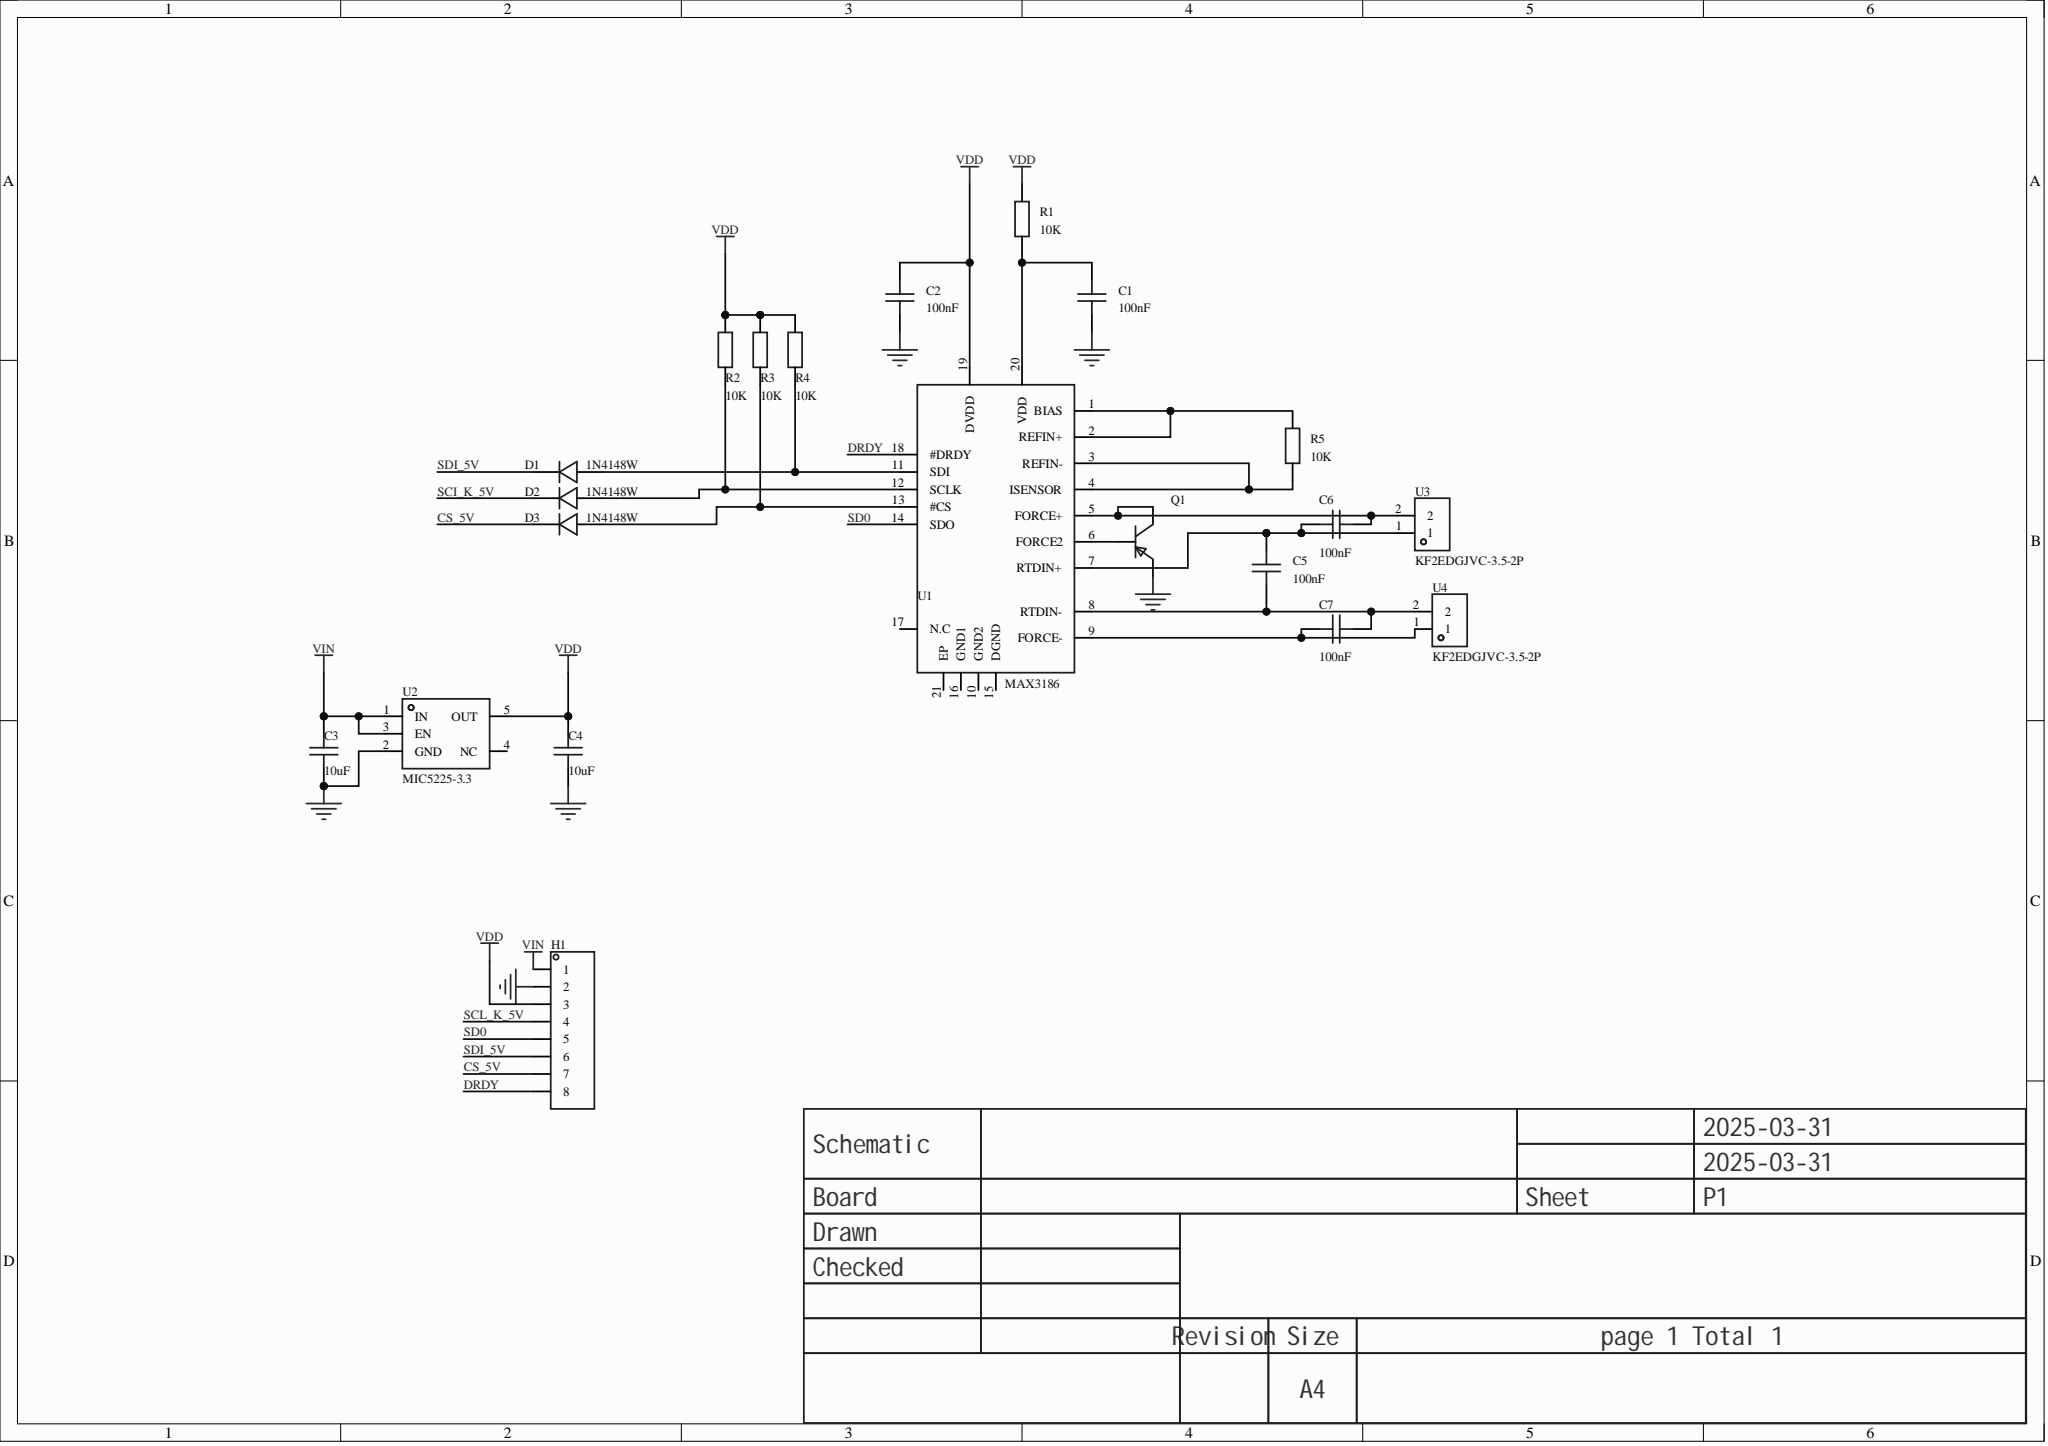Circuit board | Altium Designer | 21 parts | 18 nets
Bill of materials:
Comment,Description,Designator,Footprint,LibRef,Quantity
"100nF","","C1, C2, C5, C6, C7","C0603","CAP_0603","5"
"10uF","","C3, C4","C0603","CAP_0603","2"
"1N4148W","Diode configuration: independent; forward voltage (Vf): 1V@50mA; DC reverse voltage (Vr): 75V; rectified current: 150mA; reverse recovery time (trr): 4ns;","D1, D2, D3","SOD-123F_L2.7-W1.6-LS3.8-RD","1N4148W_C81598","3"
"","","H1","HDR-TH_8P-P2.54-V-M","HDR-M_2.54_1x8P","1"
"","","Q1","S8550P_SOT","S8550_SOT_PNP","1"
"10K","","R1, R2, R3, R4, R5","R0603","Res_0603","5"
"MAX3186","Interface: SPI; supply voltage: 3V~3.6V; sampling rate: -; resolution: 15;","U1","QFN-20_L5.0-W5.0-P0.65-BL-EP","MAX31865ATP+T","1"
"MIC5225-3.3","Output type: fixed; max input voltage: 16V; output voltage: 3.3V; output current: 150mA; output polarity: positive;","U2","SOT-23-5_L3.0-W1.7-P0.95-LS2.8-BL","MIC5225-3.3YM5-TR","1"
"KF2EDGJVC-3.5-2P","","U3, U4","CONN-TH_2P-P3.50_KEFA_KF2EDGJVC-3.5-2P","KF2EDGJVC-3.5-2P","2"
Netlist (Protel format):
[
C1
C0603
100nF



]
[
C2
C0603
100nF



]
[
C3
C0603
10uF



]
[
C4
C0603
10uF



]
[
C5
C0603
100nF



]
[
C6
C0603
100nF



]
[
C7
C0603
100nF



]
[
D1
SOD-123F_L2.7-W1.6-LS3.8-RD
1N4148W



]
[
D2
SOD-123F_L2.7-W1.6-LS3.8-RD
1N4148W



]
[
D3
SOD-123F_L2.7-W1.6-LS3.8-RD
1N4148W



]
[
H1
HDR-TH_8P-P2.54-V-M




]
[
Q1
S8550P_SOT




]
[
R1
R0603
10K



]
[
R2
R0603
10K



]
[
R3
R0603
10K



]
[
R4
R0603
10K



]
[
R5
R0603
10K



]
[
U1
QFN-20_L5.0-W5.0-P0.65-BL-EP
MAX3186



]
[
U2
SOT-23-5_L3.0-W1.7-P0.95-LS2.8-BL
MIC5225-3.3



]
[
U3
CONN-TH_2P-P3.50_KEFA_KF2EDGJVC-3.5-2P
KF2EDGJVC-3.5-2P



]
[
U4
CONN-TH_2P-P3.50_KEFA_KF2EDGJVC-3.5-2P
KF2EDGJVC-3.5-2P



]
(
VIN
C3-2
H1-1
U2-1
U2-3
)
(
VDD
C2-2
C4-2
H1-3
R1-2
R2-2
R3-2
R4-2
U1-19
U2-5
)
(
SDI_5V
D1-1
H1-6
)
(
SD0
H1-5
U1-14
)
(
NetR5_2
R5-2
U1-1
U1-2
)
(
NetR5_1
R5-1
U1-3
U1-4
)
(
NetQ1_1
Q1-1
U1-6
)
(
NetD3_2
D3-2
R3-1
U1-13
)
(
NetD2_2
D2-2
R2-1
U1-12
)
(
NetD1_2
D1-2
R4-1
U1-11
)
(
NetC7_1
C7-1
U1-9
U4-1
)
(
NetC6_2
C6-2
Q1-3
U1-5
U3-2
)
(
NetC5_2
C5-2
C6-1
U1-7
U3-1
)
(
NetC5_1
C5-1
C7-2
U1-8
U4-2
)
(
NetC1_2
C1-2
R1-1
U1-20
)
(
GND
C1-1
C2-1
C3-1
C4-1
H1-2
Q1-2
U2-2
)
(
DRDY
H1-8
U1-18
)
(
CS_5V
D3-1
H1-7
)